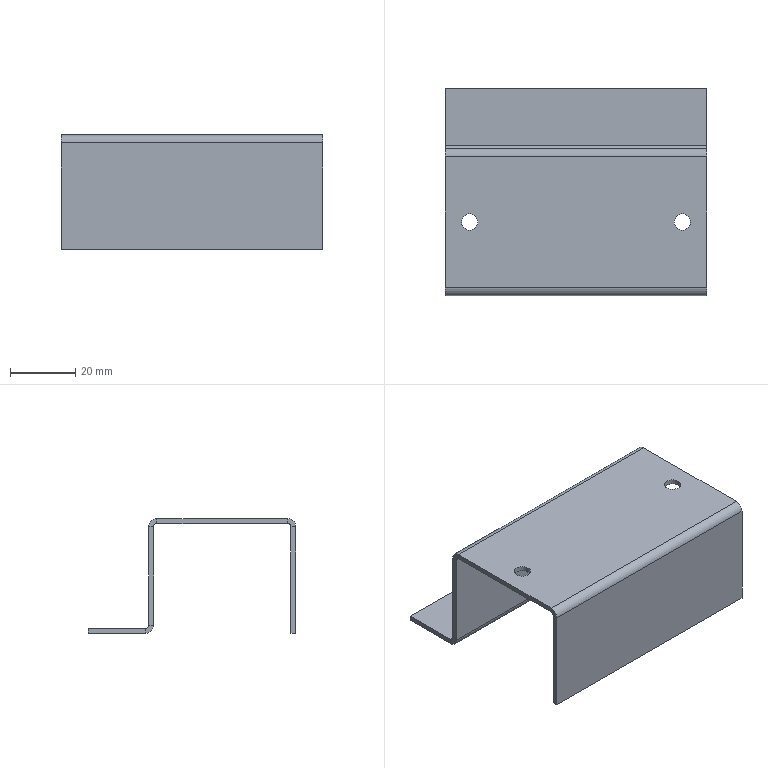Part | SolidWorks | features BaseBody 1 | 1 solid | 34 faces | box 80 x 63.5 x 35 mm | volume 15331 mm3 | plane 24 | cylinder 10 | commonest cylinder face diameters 5 x7 2 x3
STEP:
#1=CARTESIAN_POINT('',(-35.,0.,-1.5));
#2=VERTEX_POINT('',#1);
#3=CARTESIAN_POINT('',(-35.,0.,0.));
#4=VERTEX_POINT('',#3);
#5=CARTESIAN_POINT('',(-35.,0.,-1.5));
#6=DIRECTION('',(0.,0.,1.));
#7=VECTOR('',#6,1000.);
#8=LINE('',#5,#7);
#9=EDGE_CURVE('',#2,#4,#8,.T.);
#10=ORIENTED_EDGE('',*,*,#9,.F.);
#11=CARTESIAN_POINT('',(-30.,0.,-1.5));
#12=VERTEX_POINT('',#11);
#13=CARTESIAN_POINT('',(-32.5,0.,-1.5));
#14=DIRECTION('',(0.,0.,1.));
#15=DIRECTION('',(1.,0.,0.));
#16=AXIS2_PLACEMENT_3D('',#13,#14,#15);
#17=CIRCLE('',#16,2.5);
#18=EDGE_CURVE('',#12,#2,#17,.T.);
#19=ORIENTED_EDGE('',*,*,#18,.F.);
#20=CARTESIAN_POINT('',(-30.,0.,0.));
#21=VERTEX_POINT('',#20);
#22=CARTESIAN_POINT('',(-30.,0.,-1.5));
#23=DIRECTION('',(0.,0.,1.));
#24=VECTOR('',#23,1000.);
#25=LINE('',#22,#24);
#26=EDGE_CURVE('',#12,#21,#25,.T.);
#27=ORIENTED_EDGE('',*,*,#26,.T.);
#28=CARTESIAN_POINT('',(-32.5,0.,0.));
#29=DIRECTION('',(0.,0.,1.));
#30=DIRECTION('',(1.,0.,0.));
#31=AXIS2_PLACEMENT_3D('',#28,#29,#30);
#32=CIRCLE('',#31,2.5);
#33=EDGE_CURVE('',#21,#4,#32,.T.);
#34=ORIENTED_EDGE('',*,*,#33,.T.);
#35=EDGE_LOOP('',(#10,#19,#27,#34));
#36=FACE_OUTER_BOUND('',#35,.T.);
#37=CARTESIAN_POINT('',(-32.5,0.,-1.5));
#38=DIRECTION('',(0.,0.,1.));
#39=DIRECTION('',(1.,0.,0.));
#40=AXIS2_PLACEMENT_3D('',#37,#38,#39);
#41=CYLINDRICAL_SURFACE('',#40,2.5);
#42=ADVANCED_FACE('',(#36),#41,.F.);
#43=CARTESIAN_POINT('',(30.,0.,-1.5));
#44=VERTEX_POINT('',#43);
#45=CARTESIAN_POINT('',(30.,0.,0.));
#46=VERTEX_POINT('',#45);
#47=CARTESIAN_POINT('',(30.,0.,-1.5));
#48=DIRECTION('',(0.,0.,1.));
#49=VECTOR('',#48,1000.);
#50=LINE('',#47,#49);
#51=EDGE_CURVE('',#44,#46,#50,.T.);
#52=ORIENTED_EDGE('',*,*,#51,.F.);
#53=CARTESIAN_POINT('',(35.,0.,-1.5));
#54=VERTEX_POINT('',#53);
#55=CARTESIAN_POINT('',(32.5,0.,-1.5));
#56=DIRECTION('',(0.,0.,1.));
#57=DIRECTION('',(-1.,0.,0.));
#58=AXIS2_PLACEMENT_3D('',#55,#56,#57);
#59=CIRCLE('',#58,2.5);
#60=EDGE_CURVE('',#54,#44,#59,.T.);
#61=ORIENTED_EDGE('',*,*,#60,.F.);
#62=CARTESIAN_POINT('',(35.,0.,0.));
#63=VERTEX_POINT('',#62);
#64=CARTESIAN_POINT('',(35.,0.,-1.5));
#65=DIRECTION('',(0.,0.,1.));
#66=VECTOR('',#65,1000.);
#67=LINE('',#64,#66);
#68=EDGE_CURVE('',#54,#63,#67,.T.);
#69=ORIENTED_EDGE('',*,*,#68,.T.);
#70=CARTESIAN_POINT('',(32.5,0.,0.));
#71=DIRECTION('',(0.,0.,1.));
#72=DIRECTION('',(-1.,0.,0.));
#73=AXIS2_PLACEMENT_3D('',#70,#71,#72);
#74=CIRCLE('',#73,2.5);
#75=EDGE_CURVE('',#63,#46,#74,.T.);
#76=ORIENTED_EDGE('',*,*,#75,.T.);
#77=EDGE_LOOP('',(#52,#61,#69,#76));
#78=FACE_OUTER_BOUND('',#77,.T.);
#79=CARTESIAN_POINT('',(32.5,0.,-1.5));
#80=DIRECTION('',(0.,0.,1.));
#81=DIRECTION('',(1.,0.,0.));
#82=AXIS2_PLACEMENT_3D('',#79,#80,#81);
#83=CYLINDRICAL_SURFACE('',#82,2.5);
#84=ADVANCED_FACE('',(#78),#83,.F.);
#85=CARTESIAN_POINT('',(-40.,41.,-33.5));
#86=VERTEX_POINT('',#85);
#87=CARTESIAN_POINT('',(40.,41.,-33.5));
#88=VERTEX_POINT('',#87);
#89=CARTESIAN_POINT('',(40.,41.,-33.5));
#90=DIRECTION('',(1.,0.,0.));
#91=VECTOR('',#90,1000.);
#92=LINE('',#89,#91);
#93=EDGE_CURVE('',#86,#88,#92,.T.);
#94=ORIENTED_EDGE('',*,*,#93,.T.);
#95=CARTESIAN_POINT('',(40.,41.,-35.));
#96=VERTEX_POINT('',#95);
#97=CARTESIAN_POINT('',(40.,41.,-35.));
#98=DIRECTION('',(0.,0.,1.));
#99=VECTOR('',#98,1000.);
#100=LINE('',#97,#99);
#101=EDGE_CURVE('',#96,#88,#100,.T.);
#102=ORIENTED_EDGE('',*,*,#101,.F.);
#103=CARTESIAN_POINT('',(-40.,41.,-35.));
#104=VERTEX_POINT('',#103);
#105=CARTESIAN_POINT('',(0.,41.,-35.));
#106=DIRECTION('',(1.,0.,0.));
#107=VECTOR('',#106,1000.);
#108=LINE('',#105,#107);
#109=EDGE_CURVE('',#104,#96,#108,.T.);
#110=ORIENTED_EDGE('',*,*,#109,.F.);
#111=CARTESIAN_POINT('',(-40.,41.,-35.));
#112=DIRECTION('',(0.,0.,1.));
#113=VECTOR('',#112,1000.);
#114=LINE('',#111,#113);
#115=EDGE_CURVE('',#104,#86,#114,.T.);
#116=ORIENTED_EDGE('',*,*,#115,.T.);
#117=EDGE_LOOP('',(#94,#102,#110,#116));
#118=FACE_OUTER_BOUND('',#117,.T.);
#119=CARTESIAN_POINT('',(40.,41.,-35.));
#120=DIRECTION('',(0.,-1.,0.));
#121=DIRECTION('',(0.,0.,-1.));
#122=AXIS2_PLACEMENT_3D('',#119,#120,#121);
#123=PLANE('',#122);
#124=ADVANCED_FACE('',(#118),#123,.F.);
#125=CARTESIAN_POINT('',(-40.,23.5,-33.5));
#126=VERTEX_POINT('',#125);
#127=CARTESIAN_POINT('',(-40.,41.,-33.5));
#128=DIRECTION('',(0.,1.,0.));
#129=VECTOR('',#128,1000.);
#130=LINE('',#127,#129);
#131=EDGE_CURVE('',#126,#86,#130,.T.);
#132=ORIENTED_EDGE('',*,*,#131,.F.);
#133=CARTESIAN_POINT('',(40.,23.5,-33.5));
#134=VERTEX_POINT('',#133);
#135=CARTESIAN_POINT('',(40.,23.5,-33.5));
#136=DIRECTION('',(-1.,0.,0.));
#137=VECTOR('',#136,1000.);
#138=LINE('',#135,#137);
#139=EDGE_CURVE('',#134,#126,#138,.T.);
#140=ORIENTED_EDGE('',*,*,#139,.F.);
#141=CARTESIAN_POINT('',(40.,22.5,-33.5));
#142=DIRECTION('',(0.,-1.,0.));
#143=VECTOR('',#142,1000.);
#144=LINE('',#141,#143);
#145=EDGE_CURVE('',#88,#134,#144,.T.);
#146=ORIENTED_EDGE('',*,*,#145,.F.);
#147=ORIENTED_EDGE('',*,*,#93,.F.);
#148=EDGE_LOOP('',(#132,#140,#146,#147));
#149=FACE_OUTER_BOUND('',#148,.T.);
#150=CARTESIAN_POINT('',(0.,0.,-33.5));
#151=DIRECTION('',(0.,0.,1.));
#152=DIRECTION('',(1.,0.,0.));
#153=AXIS2_PLACEMENT_3D('',#150,#151,#152);
#154=PLANE('',#153);
#155=ADVANCED_FACE('',(#149),#154,.T.);
#156=CARTESIAN_POINT('',(-40.,23.5,-35.));
#157=VERTEX_POINT('',#156);
#158=CARTESIAN_POINT('',(40.,23.5,-35.));
#159=VERTEX_POINT('',#158);
#160=CARTESIAN_POINT('',(40.,23.5,-35.));
#161=DIRECTION('',(1.,0.,0.));
#162=VECTOR('',#161,1000.);
#163=LINE('',#160,#162);
#164=EDGE_CURVE('',#157,#159,#163,.T.);
#165=ORIENTED_EDGE('',*,*,#164,.F.);
#166=CARTESIAN_POINT('',(-40.,0.,-35.));
#167=DIRECTION('',(0.,1.,0.));
#168=VECTOR('',#167,1000.);
#169=LINE('',#166,#168);
#170=EDGE_CURVE('',#157,#104,#169,.T.);
#171=ORIENTED_EDGE('',*,*,#170,.T.);
#172=ORIENTED_EDGE('',*,*,#109,.T.);
#173=CARTESIAN_POINT('',(40.,0.,-35.));
#174=DIRECTION('',(0.,-1.,0.));
#175=VECTOR('',#174,1000.);
#176=LINE('',#173,#175);
#177=EDGE_CURVE('',#96,#159,#176,.T.);
#178=ORIENTED_EDGE('',*,*,#177,.T.);
#179=EDGE_LOOP('',(#165,#171,#172,#178));
#180=FACE_OUTER_BOUND('',#179,.T.);
#181=CARTESIAN_POINT('',(0.,0.,-35.));
#182=DIRECTION('',(0.,0.,1.));
#183=DIRECTION('',(1.,0.,0.));
#184=AXIS2_PLACEMENT_3D('',#181,#182,#183);
#185=PLANE('',#184);
#186=ADVANCED_FACE('',(#180),#185,.F.);
#187=CARTESIAN_POINT('',(-40.,23.5,-33.5));
#188=DIRECTION('',(0.,0.,-1.));
#189=VECTOR('',#188,1000.);
#190=LINE('',#187,#189);
#191=EDGE_CURVE('',#126,#157,#190,.T.);
#192=ORIENTED_EDGE('',*,*,#191,.F.);
#193=ORIENTED_EDGE('',*,*,#131,.T.);
#194=ORIENTED_EDGE('',*,*,#115,.F.);
#195=ORIENTED_EDGE('',*,*,#170,.F.);
#196=EDGE_LOOP('',(#192,#193,#194,#195));
#197=FACE_OUTER_BOUND('',#196,.T.);
#198=CARTESIAN_POINT('',(-40.,41.,-35.));
#199=DIRECTION('',(1.,0.,0.));
#200=DIRECTION('',(0.,1.,0.));
#201=AXIS2_PLACEMENT_3D('',#198,#199,#200);
#202=PLANE('',#201);
#203=ADVANCED_FACE('',(#197),#202,.F.);
#204=CARTESIAN_POINT('',(40.,23.5,-35.));
#205=DIRECTION('',(0.,0.,-1.));
#206=VECTOR('',#205,1000.);
#207=LINE('',#204,#206);
#208=EDGE_CURVE('',#134,#159,#207,.T.);
#209=ORIENTED_EDGE('',*,*,#208,.T.);
#210=ORIENTED_EDGE('',*,*,#177,.F.);
#211=ORIENTED_EDGE('',*,*,#101,.T.);
#212=ORIENTED_EDGE('',*,*,#145,.T.);
#213=EDGE_LOOP('',(#209,#210,#211,#212));
#214=FACE_OUTER_BOUND('',#213,.T.);
#215=CARTESIAN_POINT('',(40.,22.5,-35.));
#216=DIRECTION('',(-1.,0.,0.));
#217=DIRECTION('',(0.,0.,1.));
#218=AXIS2_PLACEMENT_3D('',#215,#216,#217);
#219=PLANE('',#218);
#220=ADVANCED_FACE('',(#214),#219,.F.);
#221=CARTESIAN_POINT('',(-40.,22.5,-32.5));
#222=VERTEX_POINT('',#221);
#223=CARTESIAN_POINT('',(40.,22.5,-32.5));
#224=VERTEX_POINT('',#223);
#225=CARTESIAN_POINT('',(-40.,22.5,-32.5));
#226=DIRECTION('',(1.,0.,0.));
#227=VECTOR('',#226,1000.);
#228=LINE('',#225,#227);
#229=EDGE_CURVE('',#222,#224,#228,.T.);
#230=ORIENTED_EDGE('',*,*,#229,.T.);
#231=CARTESIAN_POINT('',(40.,23.5,-32.5));
#232=DIRECTION('',(1.,0.,0.));
#233=DIRECTION('',(0.,0.,1.));
#234=AXIS2_PLACEMENT_3D('',#231,#232,#233);
#235=CIRCLE('',#234,1.);
#236=EDGE_CURVE('',#224,#134,#235,.T.);
#237=ORIENTED_EDGE('',*,*,#236,.T.);
#238=ORIENTED_EDGE('',*,*,#139,.T.);
#239=CARTESIAN_POINT('',(-40.,23.5,-32.5));
#240=DIRECTION('',(-1.,0.,0.));
#241=DIRECTION('',(0.,0.,1.));
#242=AXIS2_PLACEMENT_3D('',#239,#240,#241);
#243=CIRCLE('',#242,1.);
#244=EDGE_CURVE('',#126,#222,#243,.T.);
#245=ORIENTED_EDGE('',*,*,#244,.T.);
#246=EDGE_LOOP('',(#230,#237,#238,#245));
#247=FACE_OUTER_BOUND('',#246,.T.);
#248=CARTESIAN_POINT('',(-40.,23.5,-32.5));
#249=DIRECTION('',(-1.,0.,0.));
#250=DIRECTION('',(0.,0.,-1.));
#251=AXIS2_PLACEMENT_3D('',#248,#249,#250);
#252=CYLINDRICAL_SURFACE('',#251,1.);
#253=ADVANCED_FACE('',(#247),#252,.F.);
#254=CARTESIAN_POINT('',(-40.,21.,-32.5));
#255=VERTEX_POINT('',#254);
#256=CARTESIAN_POINT('',(40.,21.,-32.5));
#257=VERTEX_POINT('',#256);
#258=CARTESIAN_POINT('',(-40.,21.,-32.5));
#259=DIRECTION('',(1.,0.,0.));
#260=VECTOR('',#259,1000.);
#261=LINE('',#258,#260);
#262=EDGE_CURVE('',#255,#257,#261,.T.);
#263=ORIENTED_EDGE('',*,*,#262,.F.);
#264=CARTESIAN_POINT('',(-40.,23.5,-32.5));
#265=DIRECTION('',(-1.,0.,0.));
#266=DIRECTION('',(0.,0.,1.));
#267=AXIS2_PLACEMENT_3D('',#264,#265,#266);
#268=CIRCLE('',#267,2.5);
#269=EDGE_CURVE('',#157,#255,#268,.T.);
#270=ORIENTED_EDGE('',*,*,#269,.F.);
#271=ORIENTED_EDGE('',*,*,#164,.T.);
#272=CARTESIAN_POINT('',(40.,23.5,-32.5));
#273=DIRECTION('',(1.,0.,0.));
#274=DIRECTION('',(0.,0.,1.));
#275=AXIS2_PLACEMENT_3D('',#272,#273,#274);
#276=CIRCLE('',#275,2.5);
#277=EDGE_CURVE('',#257,#159,#276,.T.);
#278=ORIENTED_EDGE('',*,*,#277,.F.);
#279=EDGE_LOOP('',(#263,#270,#271,#278));
#280=FACE_OUTER_BOUND('',#279,.T.);
#281=CARTESIAN_POINT('',(-40.,23.5,-32.5));
#282=DIRECTION('',(-1.,0.,0.));
#283=DIRECTION('',(0.,0.,-1.));
#284=AXIS2_PLACEMENT_3D('',#281,#282,#283);
#285=CYLINDRICAL_SURFACE('',#284,2.5);
#286=ADVANCED_FACE('',(#280),#285,.T.);
#287=ORIENTED_EDGE('',*,*,#244,.F.);
#288=ORIENTED_EDGE('',*,*,#191,.T.);
#289=ORIENTED_EDGE('',*,*,#269,.T.);
#290=CARTESIAN_POINT('',(-40.,22.5,-32.5));
#291=DIRECTION('',(0.,-1.,0.));
#292=VECTOR('',#291,1000.);
#293=LINE('',#290,#292);
#294=EDGE_CURVE('',#222,#255,#293,.T.);
#295=ORIENTED_EDGE('',*,*,#294,.F.);
#296=EDGE_LOOP('',(#287,#288,#289,#295));
#297=FACE_OUTER_BOUND('',#296,.T.);
#298=CARTESIAN_POINT('',(-40.,23.5,-32.5));
#299=DIRECTION('',(1.,0.,0.));
#300=DIRECTION('',(0.,1.,0.));
#301=AXIS2_PLACEMENT_3D('',#298,#299,#300);
#302=PLANE('',#301);
#303=ADVANCED_FACE('',(#297),#302,.F.);
#304=ORIENTED_EDGE('',*,*,#208,.F.);
#305=ORIENTED_EDGE('',*,*,#236,.F.);
#306=CARTESIAN_POINT('',(40.,22.5,-32.5));
#307=DIRECTION('',(0.,-1.,0.));
#308=VECTOR('',#307,1000.);
#309=LINE('',#306,#308);
#310=EDGE_CURVE('',#224,#257,#309,.T.);
#311=ORIENTED_EDGE('',*,*,#310,.T.);
#312=ORIENTED_EDGE('',*,*,#277,.T.);
#313=EDGE_LOOP('',(#304,#305,#311,#312));
#314=FACE_OUTER_BOUND('',#313,.T.);
#315=CARTESIAN_POINT('',(40.,23.5,-32.5));
#316=DIRECTION('',(1.,0.,0.));
#317=DIRECTION('',(0.,1.,0.));
#318=AXIS2_PLACEMENT_3D('',#315,#316,#317);
#319=PLANE('',#318);
#320=ADVANCED_FACE('',(#314),#319,.T.);
#321=CARTESIAN_POINT('',(40.,20.,-1.5));
#322=VERTEX_POINT('',#321);
#323=CARTESIAN_POINT('',(-40.,20.,-1.5));
#324=VERTEX_POINT('',#323);
#325=CARTESIAN_POINT('',(40.,20.,-1.5));
#326=DIRECTION('',(-1.,0.,0.));
#327=VECTOR('',#326,1000.);
#328=LINE('',#325,#327);
#329=EDGE_CURVE('',#322,#324,#328,.T.);
#330=ORIENTED_EDGE('',*,*,#329,.T.);
#331=CARTESIAN_POINT('',(-40.,21.,-2.5));
#332=VERTEX_POINT('',#331);
#333=CARTESIAN_POINT('',(-40.,20.,-2.5));
#334=DIRECTION('',(-1.,0.,0.));
#335=DIRECTION('',(0.,0.,-1.));
#336=AXIS2_PLACEMENT_3D('',#333,#334,#335);
#337=CIRCLE('',#336,1.);
#338=EDGE_CURVE('',#324,#332,#337,.T.);
#339=ORIENTED_EDGE('',*,*,#338,.T.);
#340=CARTESIAN_POINT('',(40.,21.,-2.5));
#341=VERTEX_POINT('',#340);
#342=CARTESIAN_POINT('',(-40.,21.,-2.5));
#343=DIRECTION('',(1.,0.,0.));
#344=VECTOR('',#343,1000.);
#345=LINE('',#342,#344);
#346=EDGE_CURVE('',#332,#341,#345,.T.);
#347=ORIENTED_EDGE('',*,*,#346,.T.);
#348=CARTESIAN_POINT('',(40.,20.,-2.5));
#349=DIRECTION('',(1.,0.,0.));
#350=DIRECTION('',(0.,0.,-1.));
#351=AXIS2_PLACEMENT_3D('',#348,#349,#350);
#352=CIRCLE('',#351,1.);
#353=EDGE_CURVE('',#341,#322,#352,.T.);
#354=ORIENTED_EDGE('',*,*,#353,.T.);
#355=EDGE_LOOP('',(#330,#339,#347,#354));
#356=FACE_OUTER_BOUND('',#355,.T.);
#357=CARTESIAN_POINT('',(40.,20.,-2.5));
#358=DIRECTION('',(1.,0.,0.));
#359=DIRECTION('',(0.,1.,0.));
#360=AXIS2_PLACEMENT_3D('',#357,#358,#359);
#361=CYLINDRICAL_SURFACE('',#360,1.);
#362=ADVANCED_FACE('',(#356),#361,.F.);
#363=CARTESIAN_POINT('',(40.,20.,0.));
#364=VERTEX_POINT('',#363);
#365=CARTESIAN_POINT('',(-40.,20.,0.));
#366=VERTEX_POINT('',#365);
#367=CARTESIAN_POINT('',(40.,20.,0.));
#368=DIRECTION('',(-1.,0.,0.));
#369=VECTOR('',#368,1000.);
#370=LINE('',#367,#369);
#371=EDGE_CURVE('',#364,#366,#370,.T.);
#372=ORIENTED_EDGE('',*,*,#371,.F.);
#373=CARTESIAN_POINT('',(40.,22.5,-2.5));
#374=VERTEX_POINT('',#373);
#375=CARTESIAN_POINT('',(40.,20.,-2.5));
#376=DIRECTION('',(1.,0.,0.));
#377=DIRECTION('',(0.,0.,-1.));
#378=AXIS2_PLACEMENT_3D('',#375,#376,#377);
#379=CIRCLE('',#378,2.5);
#380=EDGE_CURVE('',#374,#364,#379,.T.);
#381=ORIENTED_EDGE('',*,*,#380,.F.);
#382=CARTESIAN_POINT('',(-40.,22.5,-2.5));
#383=VERTEX_POINT('',#382);
#384=CARTESIAN_POINT('',(-40.,22.5,-2.5));
#385=DIRECTION('',(-1.,0.,0.));
#386=VECTOR('',#385,1000.);
#387=LINE('',#384,#386);
#388=EDGE_CURVE('',#374,#383,#387,.T.);
#389=ORIENTED_EDGE('',*,*,#388,.T.);
#390=CARTESIAN_POINT('',(-40.,20.,-2.5));
#391=DIRECTION('',(-1.,0.,0.));
#392=DIRECTION('',(0.,0.,-1.));
#393=AXIS2_PLACEMENT_3D('',#390,#391,#392);
#394=CIRCLE('',#393,2.5);
#395=EDGE_CURVE('',#366,#383,#394,.T.);
#396=ORIENTED_EDGE('',*,*,#395,.F.);
#397=EDGE_LOOP('',(#372,#381,#389,#396));
#398=FACE_OUTER_BOUND('',#397,.T.);
#399=CARTESIAN_POINT('',(40.,20.,-2.5));
#400=DIRECTION('',(1.,0.,0.));
#401=DIRECTION('',(0.,1.,0.));
#402=AXIS2_PLACEMENT_3D('',#399,#400,#401);
#403=CYLINDRICAL_SURFACE('',#402,2.5);
#404=ADVANCED_FACE('',(#398),#403,.T.);
#405=ORIENTED_EDGE('',*,*,#353,.F.);
#406=CARTESIAN_POINT('',(40.,21.,-2.5));
#407=DIRECTION('',(0.,1.,0.));
#408=VECTOR('',#407,1000.);
#409=LINE('',#406,#408);
#410=EDGE_CURVE('',#341,#374,#409,.T.);
#411=ORIENTED_EDGE('',*,*,#410,.T.);
#412=ORIENTED_EDGE('',*,*,#380,.T.);
#413=CARTESIAN_POINT('',(40.,20.,-1.5));
#414=DIRECTION('',(0.,0.,1.));
#415=VECTOR('',#414,1000.);
#416=LINE('',#413,#415);
#417=EDGE_CURVE('',#322,#364,#416,.T.);
#418=ORIENTED_EDGE('',*,*,#417,.F.);
#419=EDGE_LOOP('',(#405,#411,#412,#418));
#420=FACE_OUTER_BOUND('',#419,.T.);
#421=CARTESIAN_POINT('',(40.,20.,-2.5));
#422=DIRECTION('',(-1.,0.,0.));
#423=DIRECTION('',(0.,0.,1.));
#424=AXIS2_PLACEMENT_3D('',#421,#422,#423);
#425=PLANE('',#424);
#426=ADVANCED_FACE('',(#420),#425,.F.);
#427=CARTESIAN_POINT('',(-40.,22.5,-2.5));
#428=DIRECTION('',(0.,1.,0.));
#429=VECTOR('',#428,1000.);
#430=LINE('',#427,#429);
#431=EDGE_CURVE('',#332,#383,#430,.T.);
#432=ORIENTED_EDGE('',*,*,#431,.F.);
#433=ORIENTED_EDGE('',*,*,#338,.F.);
#434=CARTESIAN_POINT('',(-40.,20.,-1.5));
#435=DIRECTION('',(0.,0.,1.));
#436=VECTOR('',#435,1000.);
#437=LINE('',#434,#436);
#438=EDGE_CURVE('',#324,#366,#437,.T.);
#439=ORIENTED_EDGE('',*,*,#438,.T.);
#440=ORIENTED_EDGE('',*,*,#395,.T.);
#441=EDGE_LOOP('',(#432,#433,#439,#440));
#442=FACE_OUTER_BOUND('',#441,.T.);
#443=CARTESIAN_POINT('',(-40.,20.,-2.5));
#444=DIRECTION('',(-1.,0.,0.));
#445=DIRECTION('',(0.,0.,1.));
#446=AXIS2_PLACEMENT_3D('',#443,#444,#445);
#447=PLANE('',#446);
#448=ADVANCED_FACE('',(#442),#447,.T.);
#449=CARTESIAN_POINT('',(-40.,-21.,-35.));
#450=VERTEX_POINT('',#449);
#451=CARTESIAN_POINT('',(40.,-21.,-35.));
#452=VERTEX_POINT('',#451);
#453=CARTESIAN_POINT('',(40.,-21.,-35.));
#454=DIRECTION('',(1.,0.,0.));
#455=VECTOR('',#454,1000.);
#456=LINE('',#453,#455);
#457=EDGE_CURVE('',#450,#452,#456,.T.);
#458=ORIENTED_EDGE('',*,*,#457,.T.);
#459=CARTESIAN_POINT('',(40.,-22.5,-35.));
#460=VERTEX_POINT('',#459);
#461=CARTESIAN_POINT('',(40.,-22.5,-35.));
#462=DIRECTION('',(0.,1.,0.));
#463=VECTOR('',#462,1000.);
#464=LINE('',#461,#463);
#465=EDGE_CURVE('',#460,#452,#464,.T.);
#466=ORIENTED_EDGE('',*,*,#465,.F.);
#467=CARTESIAN_POINT('',(-40.,-22.5,-35.));
#468=VERTEX_POINT('',#467);
#469=CARTESIAN_POINT('',(0.,-22.5,-35.));
#470=DIRECTION('',(1.,0.,0.));
#471=VECTOR('',#470,1000.);
#472=LINE('',#469,#471);
#473=EDGE_CURVE('',#468,#460,#472,.T.);
#474=ORIENTED_EDGE('',*,*,#473,.F.);
#475=CARTESIAN_POINT('',(-40.,-22.5,-35.));
#476=DIRECTION('',(0.,1.,0.));
#477=VECTOR('',#476,1000.);
#478=LINE('',#475,#477);
#479=EDGE_CURVE('',#468,#450,#478,.T.);
#480=ORIENTED_EDGE('',*,*,#479,.T.);
#481=EDGE_LOOP('',(#458,#466,#474,#480));
#482=FACE_OUTER_BOUND('',#481,.T.);
#483=CARTESIAN_POINT('',(40.,-22.5,-35.));
#484=DIRECTION('',(0.,0.,1.));
#485=DIRECTION('',(0.,-1.,0.));
#486=AXIS2_PLACEMENT_3D('',#483,#484,#485);
#487=PLANE('',#486);
#488=ADVANCED_FACE('',(#482),#487,.F.);
#489=CARTESIAN_POINT('',(-40.,-21.,-2.5));
#490=VERTEX_POINT('',#489);
#491=CARTESIAN_POINT('',(-40.,-21.,-35.));
#492=DIRECTION('',(0.,0.,-1.));
#493=VECTOR('',#492,1000.);
#494=LINE('',#491,#493);
#495=EDGE_CURVE('',#490,#450,#494,.T.);
#496=ORIENTED_EDGE('',*,*,#495,.F.);
#497=CARTESIAN_POINT('',(40.,-21.,-2.5));
#498=VERTEX_POINT('',#497);
#499=CARTESIAN_POINT('',(40.,-21.,-2.5));
#500=DIRECTION('',(-1.,0.,0.));
#501=VECTOR('',#500,1000.);
#502=LINE('',#499,#501);
#503=EDGE_CURVE('',#498,#490,#502,.T.);
#504=ORIENTED_EDGE('',*,*,#503,.F.);
#505=CARTESIAN_POINT('',(40.,-21.,-1.5));
#506=DIRECTION('',(0.,0.,1.));
#507=VECTOR('',#506,1000.);
#508=LINE('',#505,#507);
#509=EDGE_CURVE('',#452,#498,#508,.T.);
#510=ORIENTED_EDGE('',*,*,#509,.F.);
#511=ORIENTED_EDGE('',*,*,#457,.F.);
#512=EDGE_LOOP('',(#496,#504,#510,#511));
#513=FACE_OUTER_BOUND('',#512,.T.);
#514=CARTESIAN_POINT('',(0.,-21.,0.));
#515=DIRECTION('',(0.,1.,0.));
#516=DIRECTION('',(0.,0.,-1.));
#517=AXIS2_PLACEMENT_3D('',#514,#515,#516);
#518=PLANE('',#517);
#519=ADVANCED_FACE('',(#513),#518,.T.);
#520=CARTESIAN_POINT('',(-40.,-22.5,-2.5));
#521=VERTEX_POINT('',#520);
#522=CARTESIAN_POINT('',(40.,-22.5,-2.5));
#523=VERTEX_POINT('',#522);
#524=CARTESIAN_POINT('',(40.,-22.5,-2.5));
#525=DIRECTION('',(1.,0.,0.));
#526=VECTOR('',#525,1000.);
#527=LINE('',#524,#526);
#528=EDGE_CURVE('',#521,#523,#527,.T.);
#529=ORIENTED_EDGE('',*,*,#528,.F.);
#530=CARTESIAN_POINT('',(-40.,-22.5,0.));
#531=DIRECTION('',(0.,0.,-1.));
#532=VECTOR('',#531,1000.);
#533=LINE('',#530,#532);
#534=EDGE_CURVE('',#521,#468,#533,.T.);
#535=ORIENTED_EDGE('',*,*,#534,.T.);
#536=ORIENTED_EDGE('',*,*,#473,.T.);
#537=CARTESIAN_POINT('',(40.,-22.5,0.));
#538=DIRECTION('',(0.,0.,1.));
#539=VECTOR('',#538,1000.);
#540=LINE('',#537,#539);
#541=EDGE_CURVE('',#460,#523,#540,.T.);
#542=ORIENTED_EDGE('',*,*,#541,.T.);
#543=EDGE_LOOP('',(#529,#535,#536,#542));
#544=FACE_OUTER_BOUND('',#543,.T.);
#545=CARTESIAN_POINT('',(0.,-22.5,0.));
#546=DIRECTION('',(0.,1.,0.));
#547=DIRECTION('',(0.,0.,-1.));
#548=AXIS2_PLACEMENT_3D('',#545,#546,#547);
#549=PLANE('',#548);
#550=ADVANCED_FACE('',(#544),#549,.F.);
#551=CARTESIAN_POINT('',(40.,-22.5,-2.5));
#552=DIRECTION('',(0.,-1.,0.));
#553=VECTOR('',#552,1000.);
#554=LINE('',#551,#553);
#555=EDGE_CURVE('',#498,#523,#554,.T.);
#556=ORIENTED_EDGE('',*,*,#555,.T.);
#557=ORIENTED_EDGE('',*,*,#541,.F.);
#558=ORIENTED_EDGE('',*,*,#465,.T.);
#559=ORIENTED_EDGE('',*,*,#509,.T.);
#560=EDGE_LOOP('',(#556,#557,#558,#559));
#561=FACE_OUTER_BOUND('',#560,.T.);
#562=CARTESIAN_POINT('',(40.,-22.5,-1.5));
#563=DIRECTION('',(-1.,0.,0.));
#564=DIRECTION('',(0.,1.,0.));
#565=AXIS2_PLACEMENT_3D('',#562,#563,#564);
#566=PLANE('',#565);
#567=ADVANCED_FACE('',(#561),#566,.F.);
#568=CARTESIAN_POINT('',(-40.,-21.,-2.5));
#569=DIRECTION('',(0.,-1.,0.));
#570=VECTOR('',#569,1000.);
#571=LINE('',#568,#570);
#572=EDGE_CURVE('',#490,#521,#571,.T.);
#573=ORIENTED_EDGE('',*,*,#572,.F.);
#574=ORIENTED_EDGE('',*,*,#495,.T.);
#575=ORIENTED_EDGE('',*,*,#479,.F.);
#576=ORIENTED_EDGE('',*,*,#534,.F.);
#577=EDGE_LOOP('',(#573,#574,#575,#576));
#578=FACE_OUTER_BOUND('',#577,.T.);
#579=CARTESIAN_POINT('',(-40.,-22.5,-35.));
#580=DIRECTION('',(1.,0.,0.));
#581=DIRECTION('',(0.,1.,0.));
#582=AXIS2_PLACEMENT_3D('',#579,#580,#581);
#583=PLANE('',#582);
#584=ADVANCED_FACE('',(#578),#583,.F.);
#585=CARTESIAN_POINT('',(-40.,-20.,-1.5));
#586=VERTEX_POINT('',#585);
#587=CARTESIAN_POINT('',(40.,-20.,-1.5));
#588=VERTEX_POINT('',#587);
#589=CARTESIAN_POINT('',(-40.,-20.,-1.5));
#590=DIRECTION('',(1.,0.,0.));
#591=VECTOR('',#590,1000.);
#592=LINE('',#589,#591);
#593=EDGE_CURVE('',#586,#588,#592,.T.);
#594=ORIENTED_EDGE('',*,*,#593,.T.);
#595=CARTESIAN_POINT('',(40.,-20.,-2.5));
#596=DIRECTION('',(1.,0.,0.));
#597=DIRECTION('',(0.,0.,1.));
#598=AXIS2_PLACEMENT_3D('',#595,#596,#597);
#599=CIRCLE('',#598,1.);
#600=EDGE_CURVE('',#588,#498,#599,.T.);
#601=ORIENTED_EDGE('',*,*,#600,.T.);
#602=ORIENTED_EDGE('',*,*,#503,.T.);
#603=CARTESIAN_POINT('',(-40.,-20.,-2.5));
#604=DIRECTION('',(-1.,0.,0.));
#605=DIRECTION('',(0.,0.,1.));
#606=AXIS2_PLACEMENT_3D('',#603,#604,#605);
#607=CIRCLE('',#606,1.);
#608=EDGE_CURVE('',#490,#586,#607,.T.);
#609=ORIENTED_EDGE('',*,*,#608,.T.);
#610=EDGE_LOOP('',(#594,#601,#602,#609));
#611=FACE_OUTER_BOUND('',#610,.T.);
#612=CARTESIAN_POINT('',(-40.,-20.,-2.5));
#613=DIRECTION('',(-1.,0.,0.));
#614=DIRECTION('',(0.,-1.,0.));
#615=AXIS2_PLACEMENT_3D('',#612,#613,#614);
#616=CYLINDRICAL_SURFACE('',#615,1.);
#617=ADVANCED_FACE('',(#611),#616,.F.);
#618=CARTESIAN_POINT('',(-40.,-20.,0.));
#619=VERTEX_POINT('',#618);
#620=CARTESIAN_POINT('',(40.,-20.,0.));
#621=VERTEX_POINT('',#620);
#622=CARTESIAN_POINT('',(-40.,-20.,0.));
#623=DIRECTION('',(1.,0.,0.));
#624=VECTOR('',#623,1000.);
#625=LINE('',#622,#624);
#626=EDGE_CURVE('',#619,#621,#625,.T.);
#627=ORIENTED_EDGE('',*,*,#626,.F.);
#628=CARTESIAN_POINT('',(-40.,-20.,-2.5));
#629=DIRECTION('',(-1.,0.,0.));
#630=DIRECTION('',(0.,0.,1.));
#631=AXIS2_PLACEMENT_3D('',#628,#629,#630);
#632=CIRCLE('',#631,2.5);
#633=EDGE_CURVE('',#521,#619,#632,.T.);
#634=ORIENTED_EDGE('',*,*,#633,.F.);
#635=ORIENTED_EDGE('',*,*,#528,.T.);
#636=CARTESIAN_POINT('',(40.,-20.,-2.5));
#637=DIRECTION('',(1.,0.,0.));
#638=DIRECTION('',(0.,0.,1.));
#639=AXIS2_PLACEMENT_3D('',#636,#637,#638);
#640=CIRCLE('',#639,2.5);
#641=EDGE_CURVE('',#621,#523,#640,.T.);
#642=ORIENTED_EDGE('',*,*,#641,.F.);
#643=EDGE_LOOP('',(#627,#634,#635,#642));
#644=FACE_OUTER_BOUND('',#643,.T.);
#645=CARTESIAN_POINT('',(-40.,-20.,-2.5));
#646=DIRECTION('',(-1.,0.,0.));
#647=DIRECTION('',(0.,-1.,0.));
#648=AXIS2_PLACEMENT_3D('',#645,#646,#647);
#649=CYLINDRICAL_SURFACE('',#648,2.5);
#650=ADVANCED_FACE('',(#644),#649,.T.);
#651=ORIENTED_EDGE('',*,*,#608,.F.);
#652=ORIENTED_EDGE('',*,*,#572,.T.);
#653=ORIENTED_EDGE('',*,*,#633,.T.);
#654=CARTESIAN_POINT('',(-40.,-20.,-1.5));
#655=DIRECTION('',(0.,0.,1.));
#656=VECTOR('',#655,1000.);
#657=LINE('',#654,#656);
#658=EDGE_CURVE('',#586,#619,#657,.T.);
#659=ORIENTED_EDGE('',*,*,#658,.F.);
#660=EDGE_LOOP('',(#651,#652,#653,#659));
#661=FACE_OUTER_BOUND('',#660,.T.);
#662=CARTESIAN_POINT('',(-40.,-20.,-2.5));
#663=DIRECTION('',(1.,0.,0.));
#664=DIRECTION('',(0.,0.,-1.));
#665=AXIS2_PLACEMENT_3D('',#662,#663,#664);
#666=PLANE('',#665);
#667=ADVANCED_FACE('',(#661),#666,.F.);
#668=ORIENTED_EDGE('',*,*,#555,.F.);
#669=ORIENTED_EDGE('',*,*,#600,.F.);
#670=CARTESIAN_POINT('',(40.,-20.,-1.5));
#671=DIRECTION('',(0.,0.,1.));
#672=VECTOR('',#671,1000.);
#673=LINE('',#670,#672);
#674=EDGE_CURVE('',#588,#621,#673,.T.);
#675=ORIENTED_EDGE('',*,*,#674,.T.);
#676=ORIENTED_EDGE('',*,*,#641,.T.);
#677=EDGE_LOOP('',(#668,#669,#675,#676));
#678=FACE_OUTER_BOUND('',#677,.T.);
#679=CARTESIAN_POINT('',(40.,-20.,-2.5));
#680=DIRECTION('',(1.,0.,0.));
#681=DIRECTION('',(0.,0.,-1.));
#682=AXIS2_PLACEMENT_3D('',#679,#680,#681);
#683=PLANE('',#682);
#684=ADVANCED_FACE('',(#678),#683,.T.);
#685=ORIENTED_EDGE('',*,*,#438,.F.);
#686=CARTESIAN_POINT('',(-40.,22.5,-1.5));
#687=DIRECTION('',(0.,-1.,0.));
#688=VECTOR('',#687,1000.);
#689=LINE('',#686,#688);
#690=EDGE_CURVE('',#324,#586,#689,.T.);
#691=ORIENTED_EDGE('',*,*,#690,.T.);
#692=ORIENTED_EDGE('',*,*,#658,.T.);
#693=CARTESIAN_POINT('',(-40.,22.5,0.));
#694=DIRECTION('',(0.,-1.,0.));
#695=VECTOR('',#694,1000.);
#696=LINE('',#693,#695);
#697=EDGE_CURVE('',#366,#619,#696,.T.);
#698=ORIENTED_EDGE('',*,*,#697,.F.);
#699=EDGE_LOOP('',(#685,#691,#692,#698));
#700=FACE_OUTER_BOUND('',#699,.T.);
#701=CARTESIAN_POINT('',(-40.,22.5,-1.5));
#702=DIRECTION('',(-1.,0.,0.));
#703=DIRECTION('',(0.,0.,1.));
#704=AXIS2_PLACEMENT_3D('',#701,#702,#703);
#705=PLANE('',#704);
#706=ADVANCED_FACE('',(#700),#705,.T.);
#707=CARTESIAN_POINT('',(40.,22.5,-1.5));
#708=DIRECTION('',(0.,1.,0.));
#709=VECTOR('',#708,1000.);
#710=LINE('',#707,#709);
#711=EDGE_CURVE('',#588,#322,#710,.T.);
#712=ORIENTED_EDGE('',*,*,#711,.T.);
#713=ORIENTED_EDGE('',*,*,#417,.T.);
#714=CARTESIAN_POINT('',(40.,22.5,0.));
#715=DIRECTION('',(0.,1.,0.));
#716=VECTOR('',#715,1000.);
#717=LINE('',#714,#716);
#718=EDGE_CURVE('',#621,#364,#717,.T.);
#719=ORIENTED_EDGE('',*,*,#718,.F.);
#720=ORIENTED_EDGE('',*,*,#674,.F.);
#721=EDGE_LOOP('',(#712,#713,#719,#720));
#722=FACE_OUTER_BOUND('',#721,.T.);
#723=CARTESIAN_POINT('',(40.,22.5,-1.5));
#724=DIRECTION('',(1.,0.,0.));
#725=DIRECTION('',(0.,1.,0.));
#726=AXIS2_PLACEMENT_3D('',#723,#724,#725);
#727=PLANE('',#726);
#728=ADVANCED_FACE('',(#722),#727,.T.);
#729=ORIENTED_EDGE('',*,*,#75,.F.);
#730=CARTESIAN_POINT('',(32.5,0.,0.));
#731=DIRECTION('',(0.,0.,1.));
#732=DIRECTION('',(-1.,0.,0.));
#733=AXIS2_PLACEMENT_3D('',#730,#731,#732);
#734=CIRCLE('',#733,2.5);
#735=EDGE_CURVE('',#46,#63,#734,.T.);
#736=ORIENTED_EDGE('',*,*,#735,.F.);
#737=EDGE_LOOP('',(#729,#736));
#738=FACE_BOUND('',#737,.T.);
#739=ORIENTED_EDGE('',*,*,#33,.F.);
#740=CARTESIAN_POINT('',(-32.5,0.,0.));
#741=DIRECTION('',(0.,0.,1.));
#742=DIRECTION('',(1.,0.,0.));
#743=AXIS2_PLACEMENT_3D('',#740,#741,#742);
#744=CIRCLE('',#743,2.5);
#745=EDGE_CURVE('',#4,#21,#744,.T.);
#746=ORIENTED_EDGE('',*,*,#745,.F.);
#747=EDGE_LOOP('',(#739,#746));
#748=FACE_BOUND('',#747,.T.);
#749=ORIENTED_EDGE('',*,*,#371,.T.);
#750=ORIENTED_EDGE('',*,*,#697,.T.);
#751=ORIENTED_EDGE('',*,*,#626,.T.);
#752=ORIENTED_EDGE('',*,*,#718,.T.);
#753=EDGE_LOOP('',(#749,#750,#751,#752));
#754=FACE_OUTER_BOUND('',#753,.T.);
#755=CARTESIAN_POINT('',(0.,0.,0.));
#756=DIRECTION('',(0.,0.,-1.));
#757=DIRECTION('',(0.,-1.,0.));
#758=AXIS2_PLACEMENT_3D('',#755,#756,#757);
#759=PLANE('',#758);
#760=ADVANCED_FACE('',(#738,#748,#754),#759,.F.);
#761=ORIENTED_EDGE('',*,*,#60,.T.);
#762=CARTESIAN_POINT('',(32.5,0.,-1.5));
#763=DIRECTION('',(0.,0.,1.));
#764=DIRECTION('',(-1.,0.,0.));
#765=AXIS2_PLACEMENT_3D('',#762,#763,#764);
#766=CIRCLE('',#765,2.5);
#767=EDGE_CURVE('',#44,#54,#766,.T.);
#768=ORIENTED_EDGE('',*,*,#767,.T.);
#769=EDGE_LOOP('',(#761,#768));
#770=FACE_BOUND('',#769,.T.);
#771=ORIENTED_EDGE('',*,*,#18,.T.);
#772=CARTESIAN_POINT('',(-32.5,0.,-1.5));
#773=DIRECTION('',(0.,0.,1.));
#774=DIRECTION('',(1.,0.,0.));
#775=AXIS2_PLACEMENT_3D('',#772,#773,#774);
#776=CIRCLE('',#775,2.5);
#777=EDGE_CURVE('',#2,#12,#776,.T.);
#778=ORIENTED_EDGE('',*,*,#777,.T.);
#779=EDGE_LOOP('',(#771,#778));
#780=FACE_BOUND('',#779,.T.);
#781=ORIENTED_EDGE('',*,*,#690,.F.);
#782=ORIENTED_EDGE('',*,*,#329,.F.);
#783=ORIENTED_EDGE('',*,*,#711,.F.);
#784=ORIENTED_EDGE('',*,*,#593,.F.);
#785=EDGE_LOOP('',(#781,#782,#783,#784));
#786=FACE_OUTER_BOUND('',#785,.T.);
#787=CARTESIAN_POINT('',(0.,0.,-1.5));
#788=DIRECTION('',(0.,0.,-1.));
#789=DIRECTION('',(0.,-1.,0.));
#790=AXIS2_PLACEMENT_3D('',#787,#788,#789);
#791=PLANE('',#790);
#792=ADVANCED_FACE('',(#770,#780,#786),#791,.T.);
#793=CARTESIAN_POINT('',(-40.,21.,-1.5));
#794=DIRECTION('',(0.,0.,1.));
#795=VECTOR('',#794,1000.);
#796=LINE('',#793,#795);
#797=EDGE_CURVE('',#255,#332,#796,.T.);
#798=ORIENTED_EDGE('',*,*,#797,.F.);
#799=ORIENTED_EDGE('',*,*,#262,.T.);
#800=CARTESIAN_POINT('',(40.,21.,-35.));
#801=DIRECTION('',(0.,0.,-1.));
#802=VECTOR('',#801,1000.);
#803=LINE('',#800,#802);
#804=EDGE_CURVE('',#341,#257,#803,.T.);
#805=ORIENTED_EDGE('',*,*,#804,.F.);
#806=ORIENTED_EDGE('',*,*,#346,.F.);
#807=EDGE_LOOP('',(#798,#799,#805,#806));
#808=FACE_OUTER_BOUND('',#807,.T.);
#809=CARTESIAN_POINT('',(0.,21.,0.));
#810=DIRECTION('',(0.,-1.,0.));
#811=DIRECTION('',(0.,0.,-1.));
#812=AXIS2_PLACEMENT_3D('',#809,#810,#811);
#813=PLANE('',#812);
#814=ADVANCED_FACE('',(#808),#813,.T.);
#815=ORIENTED_EDGE('',*,*,#229,.F.);
#816=CARTESIAN_POINT('',(-40.,22.5,0.));
#817=DIRECTION('',(0.,0.,1.));
#818=VECTOR('',#817,1000.);
#819=LINE('',#816,#818);
#820=EDGE_CURVE('',#222,#383,#819,.T.);
#821=ORIENTED_EDGE('',*,*,#820,.T.);
#822=ORIENTED_EDGE('',*,*,#388,.F.);
#823=CARTESIAN_POINT('',(40.,22.5,0.));
#824=DIRECTION('',(0.,0.,-1.));
#825=VECTOR('',#824,1000.);
#826=LINE('',#823,#825);
#827=EDGE_CURVE('',#374,#224,#826,.T.);
#828=ORIENTED_EDGE('',*,*,#827,.T.);
#829=EDGE_LOOP('',(#815,#821,#822,#828));
#830=FACE_OUTER_BOUND('',#829,.T.);
#831=CARTESIAN_POINT('',(0.,22.5,0.));
#832=DIRECTION('',(0.,-1.,0.));
#833=DIRECTION('',(0.,0.,-1.));
#834=AXIS2_PLACEMENT_3D('',#831,#832,#833);
#835=PLANE('',#834);
#836=ADVANCED_FACE('',(#830),#835,.F.);
#837=ORIENTED_EDGE('',*,*,#294,.T.);
#838=ORIENTED_EDGE('',*,*,#797,.T.);
#839=ORIENTED_EDGE('',*,*,#431,.T.);
#840=ORIENTED_EDGE('',*,*,#820,.F.);
#841=EDGE_LOOP('',(#837,#838,#839,#840));
#842=FACE_OUTER_BOUND('',#841,.T.);
#843=CARTESIAN_POINT('',(-40.,22.5,-1.5));
#844=DIRECTION('',(1.,0.,0.));
#845=DIRECTION('',(0.,0.,-1.));
#846=AXIS2_PLACEMENT_3D('',#843,#844,#845);
#847=PLANE('',#846);
#848=ADVANCED_FACE('',(#842),#847,.F.);
#849=ORIENTED_EDGE('',*,*,#310,.F.);
#850=ORIENTED_EDGE('',*,*,#827,.F.);
#851=ORIENTED_EDGE('',*,*,#410,.F.);
#852=ORIENTED_EDGE('',*,*,#804,.T.);
#853=EDGE_LOOP('',(#849,#850,#851,#852));
#854=FACE_OUTER_BOUND('',#853,.T.);
#855=CARTESIAN_POINT('',(40.,22.5,-35.));
#856=DIRECTION('',(-1.,0.,0.));
#857=DIRECTION('',(0.,1.,0.));
#858=AXIS2_PLACEMENT_3D('',#855,#856,#857);
#859=PLANE('',#858);
#860=ADVANCED_FACE('',(#854),#859,.F.);
#861=ORIENTED_EDGE('',*,*,#767,.F.);
#862=ORIENTED_EDGE('',*,*,#51,.T.);
#863=ORIENTED_EDGE('',*,*,#735,.T.);
#864=ORIENTED_EDGE('',*,*,#68,.F.);
#865=EDGE_LOOP('',(#861,#862,#863,#864));
#866=FACE_OUTER_BOUND('',#865,.T.);
#867=CARTESIAN_POINT('',(32.5,0.,-1.5));
#868=DIRECTION('',(0.,0.,1.));
#869=DIRECTION('',(1.,0.,0.));
#870=AXIS2_PLACEMENT_3D('',#867,#868,#869);
#871=CYLINDRICAL_SURFACE('',#870,2.5);
#872=ADVANCED_FACE('',(#866),#871,.F.);
#873=ORIENTED_EDGE('',*,*,#777,.F.);
#874=ORIENTED_EDGE('',*,*,#9,.T.);
#875=ORIENTED_EDGE('',*,*,#745,.T.);
#876=ORIENTED_EDGE('',*,*,#26,.F.);
#877=EDGE_LOOP('',(#873,#874,#875,#876));
#878=FACE_OUTER_BOUND('',#877,.T.);
#879=CARTESIAN_POINT('',(-32.5,0.,-1.5));
#880=DIRECTION('',(0.,0.,1.));
#881=DIRECTION('',(1.,0.,0.));
#882=AXIS2_PLACEMENT_3D('',#879,#880,#881);
#883=CYLINDRICAL_SURFACE('',#882,2.5);
#884=ADVANCED_FACE('',(#878),#883,.F.);
#885=CLOSED_SHELL('',(#42,#84,#124,#155,#186,#203,#220,#253,#286,#303,#320,#362,#404,#426,#448,#488,#519,#550,#567,#584,#617,#650,#667,#684,#706,#728,#760,#792,#814,#836,#848,#860,#872,#884));
#886=MANIFOLD_SOLID_BREP('',#885);
#887=CARTESIAN_POINT('',(0.,0.,0.));
#888=DIRECTION('',(0.,0.,1.));
#889=DIRECTION('',(1.,0.,0.));
#890=AXIS2_PLACEMENT_3D('',#887,#888,#889);
#891=(LENGTH_UNIT()NAMED_UNIT(*)SI_UNIT(.MILLI.,.METRE.));
#892=UNCERTAINTY_MEASURE_WITH_UNIT(LENGTH_MEASURE(0.00001),#891,'','');
#893=(NAMED_UNIT(*)PLANE_ANGLE_UNIT()SI_UNIT($,.RADIAN.));
#894=(NAMED_UNIT(*)SI_UNIT($,.STERADIAN.)SOLID_ANGLE_UNIT());
#895=(GEOMETRIC_REPRESENTATION_CONTEXT(3)GLOBAL_UNCERTAINTY_ASSIGNED_CONTEXT((#892))GLOBAL_UNIT_ASSIGNED_CONTEXT((#891,#893,#894))REPRESENTATION_CONTEXT('',''));
#896=ADVANCED_BREP_SHAPE_REPRESENTATION('',(#886,#890),#895);